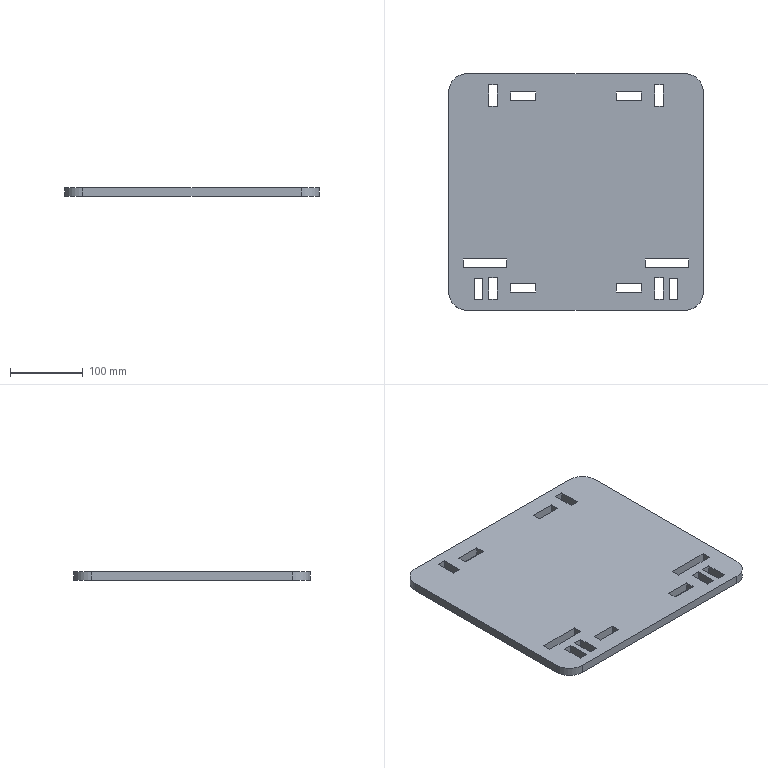Part | SolidWorks | features FlatPattern 1, SMBaseFlange 1, SheetMetal 1 | 1 solid | 58 faces | box 350 x 325 x 12 mm | volume 1295202 mm3 | plane 54 | cylinder 4 | commonest cylinder face diameters 50 x4